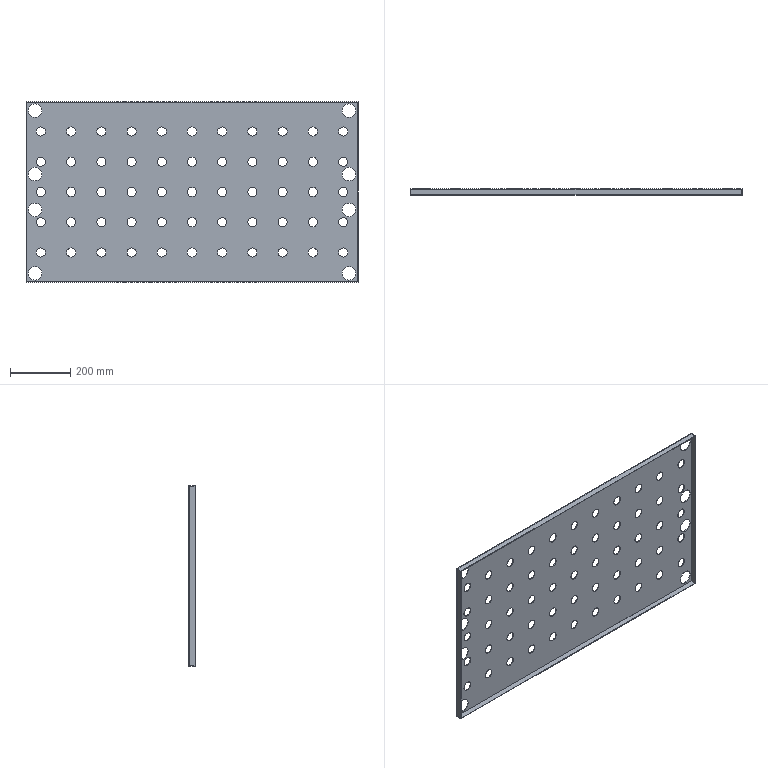Part | NX | 1 solid | 74 faces | box 1098 x 20 x 598 mm | volume 1331831 mm3 | cylinder 63 | plane 11 | commonest cylinder face diameters 30 x55 45 x8